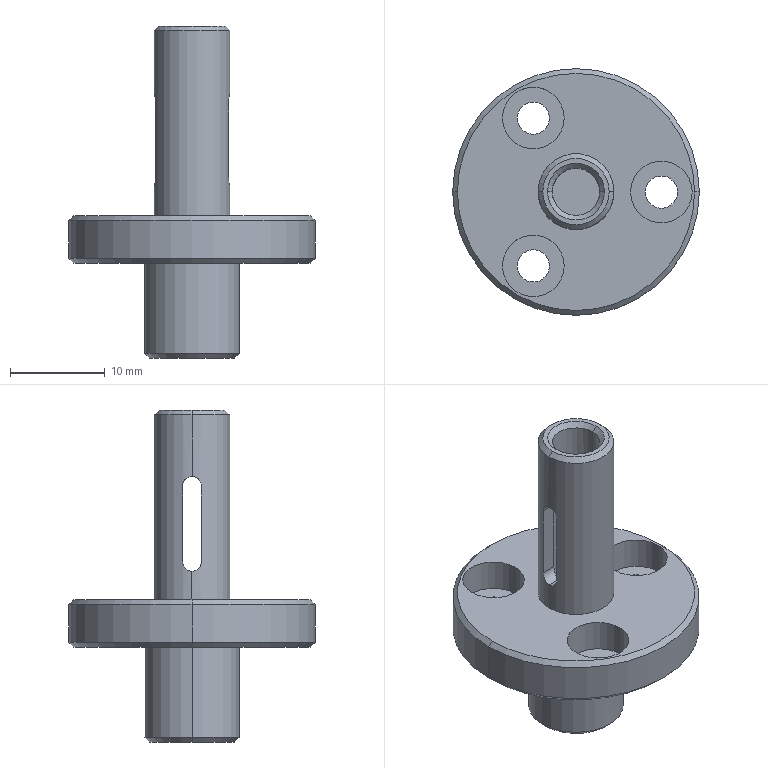Part | SolidWorks | features ICE 4, Chamfer 1, CirPattern 1, Extrusion 1, HoleWzd 1 | 1 solid | 48 faces | box 26 x 26 x 35 mm | volume 3387 mm3 | cylinder 26 | plane 12 | cone 10 | commonest cylinder face diameters 2 x6 3.4 x6 6.5 x6 5 x2 8 x2 10 x2